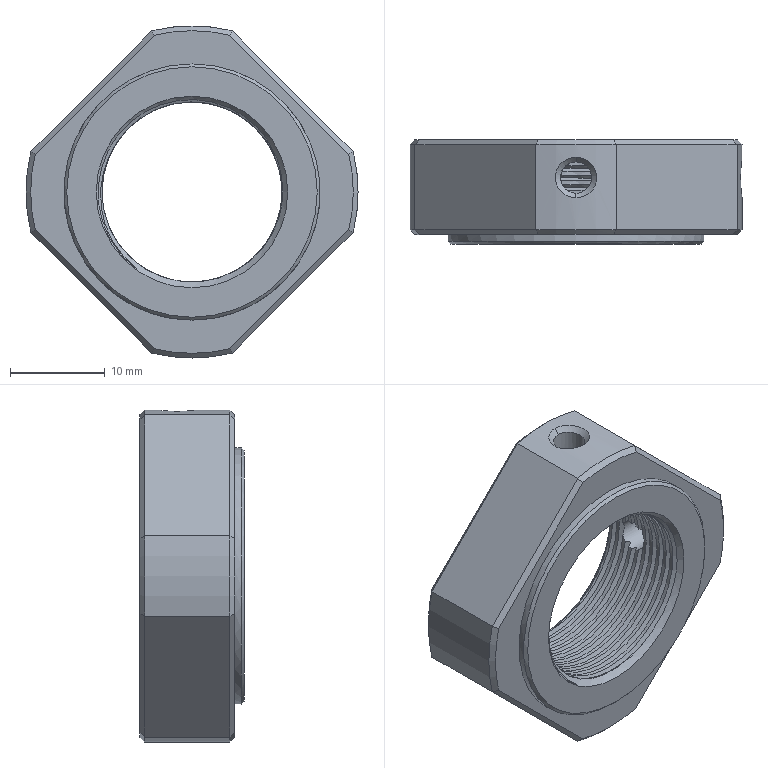Part | STEP file | BK-20_id1206_x_t | 1 solid | 58 faces | box 35 x 11 x 35 mm | volume 5569 mm3 | spline 18 | plane 15 | cylinder 14 | cone 11 | commonest cylinder face diameters 19 x7 35 x4 3.3 x2 27 x1